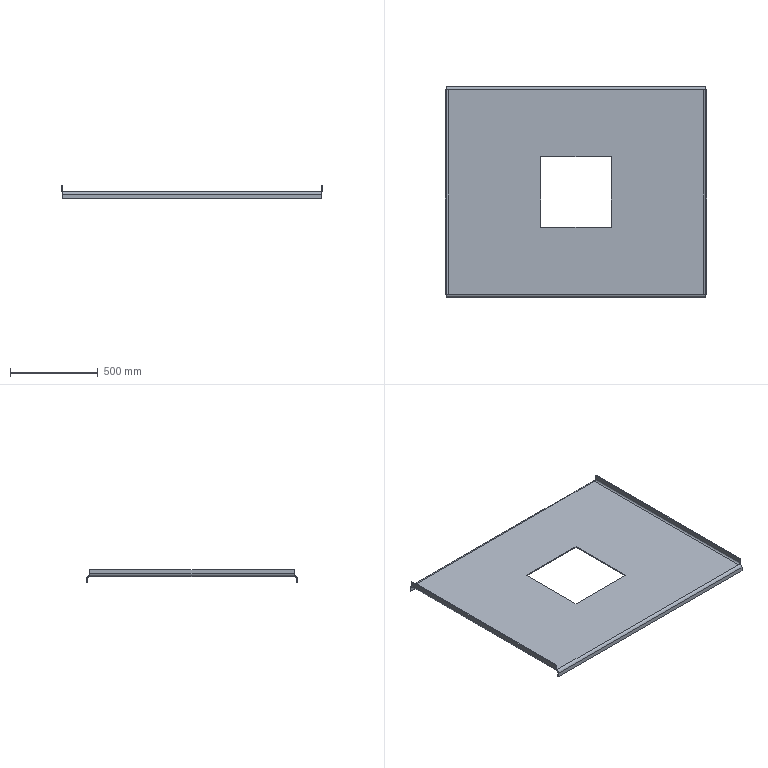Part | SolidWorks | features EdgeFlange 2, FlatPattern 1, ICE 1, SMBaseFlange 1, SheetMetal 1 | 1 solid | 46 faces | box 1492 x 1200 x 74 mm | volume 10683181 mm3 | plane 38 | cylinder 8 | commonest cylinder face diameters 20 x4 32 x4
STEP:
#1=CARTESIAN_POINT('',(740.,584.,-6.));
#2=VERTEX_POINT('',#1);
#3=CARTESIAN_POINT('',(740.,584.,-2.49));
#4=VERTEX_POINT('',#3);
#5=CARTESIAN_POINT('',(740.,584.,-6.));
#6=DIRECTION('',(0.,0.,1.));
#7=VECTOR('',#6,1000.);
#8=LINE('',#5,#7);
#9=EDGE_CURVE('',#2,#4,#8,.T.);
#10=ORIENTED_EDGE('',*,*,#9,.T.);
#11=CARTESIAN_POINT('',(730.,584.,-6.));
#12=VERTEX_POINT('',#11);
#13=CARTESIAN_POINT('',(730.,584.,10.));
#14=DIRECTION('',(0.,1.,0.));
#15=DIRECTION('',(0.,0.,1.));
#16=AXIS2_PLACEMENT_3D('',#13,#14,#15);
#17=CIRCLE('',#16,16.);
#18=EDGE_CURVE('',#4,#12,#17,.T.);
#19=ORIENTED_EDGE('',*,*,#18,.T.);
#20=CARTESIAN_POINT('',(740.,584.,-6.));
#21=DIRECTION('',(-1.,0.,0.));
#22=VECTOR('',#21,1000.);
#23=LINE('',#20,#22);
#24=EDGE_CURVE('',#2,#12,#23,.T.);
#25=ORIENTED_EDGE('',*,*,#24,.F.);
#26=EDGE_LOOP('',(#10,#19,#25));
#27=FACE_OUTER_BOUND('',#26,.T.);
#28=CARTESIAN_POINT('',(740.,584.,0.));
#29=DIRECTION('',(0.,-1.,0.));
#30=DIRECTION('',(1.,0.,0.));
#31=AXIS2_PLACEMENT_3D('',#28,#29,#30);
#32=PLANE('',#31);
#33=ADVANCED_FACE('',(#27),#32,.T.);
#34=CARTESIAN_POINT('',(730.,-584.,-6.));
#35=VERTEX_POINT('',#34);
#36=CARTESIAN_POINT('',(740.,-584.,-6.));
#37=VERTEX_POINT('',#36);
#38=CARTESIAN_POINT('',(-740.,-584.,-6.));
#39=DIRECTION('',(1.,0.,0.));
#40=VECTOR('',#39,1000.);
#41=LINE('',#38,#40);
#42=EDGE_CURVE('',#35,#37,#41,.T.);
#43=ORIENTED_EDGE('',*,*,#42,.F.);
#44=CARTESIAN_POINT('',(740.,-584.,-2.49));
#45=VERTEX_POINT('',#44);
#46=CARTESIAN_POINT('',(730.,-584.,10.));
#47=DIRECTION('',(0.,-1.,0.));
#48=DIRECTION('',(0.,0.,1.));
#49=AXIS2_PLACEMENT_3D('',#46,#47,#48);
#50=CIRCLE('',#49,16.);
#51=EDGE_CURVE('',#35,#45,#50,.T.);
#52=ORIENTED_EDGE('',*,*,#51,.T.);
#53=CARTESIAN_POINT('',(740.,-584.,-6.));
#54=DIRECTION('',(0.,0.,1.));
#55=VECTOR('',#54,1000.);
#56=LINE('',#53,#55);
#57=EDGE_CURVE('',#37,#45,#56,.T.);
#58=ORIENTED_EDGE('',*,*,#57,.F.);
#59=EDGE_LOOP('',(#43,#52,#58));
#60=FACE_OUTER_BOUND('',#59,.T.);
#61=CARTESIAN_POINT('',(730.,-584.,0.));
#62=DIRECTION('',(0.,1.,0.));
#63=DIRECTION('',(0.,0.,1.));
#64=AXIS2_PLACEMENT_3D('',#61,#62,#63);
#65=PLANE('',#64);
#66=ADVANCED_FACE('',(#60),#65,.T.);
#67=CARTESIAN_POINT('',(-740.,-584.,-6.));
#68=VERTEX_POINT('',#67);
#69=CARTESIAN_POINT('',(-740.,-584.,-2.49));
#70=VERTEX_POINT('',#69);
#71=CARTESIAN_POINT('',(-740.,-584.,-6.));
#72=DIRECTION('',(0.,0.,1.));
#73=VECTOR('',#72,1000.);
#74=LINE('',#71,#73);
#75=EDGE_CURVE('',#68,#70,#74,.T.);
#76=ORIENTED_EDGE('',*,*,#75,.T.);
#77=CARTESIAN_POINT('',(-730.,-584.,-6.));
#78=VERTEX_POINT('',#77);
#79=CARTESIAN_POINT('',(-730.,-584.,10.));
#80=DIRECTION('',(0.,-1.,0.));
#81=DIRECTION('',(0.,0.,-1.));
#82=AXIS2_PLACEMENT_3D('',#79,#80,#81);
#83=CIRCLE('',#82,16.);
#84=EDGE_CURVE('',#70,#78,#83,.T.);
#85=ORIENTED_EDGE('',*,*,#84,.T.);
#86=CARTESIAN_POINT('',(-740.,-584.,-6.));
#87=DIRECTION('',(1.,0.,0.));
#88=VECTOR('',#87,1000.);
#89=LINE('',#86,#88);
#90=EDGE_CURVE('',#68,#78,#89,.T.);
#91=ORIENTED_EDGE('',*,*,#90,.F.);
#92=EDGE_LOOP('',(#76,#85,#91));
#93=FACE_OUTER_BOUND('',#92,.T.);
#94=CARTESIAN_POINT('',(-740.,-584.,0.));
#95=DIRECTION('',(0.,1.,0.));
#96=DIRECTION('',(-1.,0.,0.));
#97=AXIS2_PLACEMENT_3D('',#94,#95,#96);
#98=PLANE('',#97);
#99=ADVANCED_FACE('',(#93),#98,.T.);
#100=CARTESIAN_POINT('',(-730.,584.,-6.));
#101=VERTEX_POINT('',#100);
#102=CARTESIAN_POINT('',(-740.,584.,-6.));
#103=VERTEX_POINT('',#102);
#104=CARTESIAN_POINT('',(740.,584.,-6.));
#105=DIRECTION('',(-1.,0.,0.));
#106=VECTOR('',#105,1000.);
#107=LINE('',#104,#106);
#108=EDGE_CURVE('',#101,#103,#107,.T.);
#109=ORIENTED_EDGE('',*,*,#108,.F.);
#110=CARTESIAN_POINT('',(-740.,584.,-2.49));
#111=VERTEX_POINT('',#110);
#112=CARTESIAN_POINT('',(-730.,584.,10.));
#113=DIRECTION('',(0.,1.,0.));
#114=DIRECTION('',(0.,0.,-1.));
#115=AXIS2_PLACEMENT_3D('',#112,#113,#114);
#116=CIRCLE('',#115,16.);
#117=EDGE_CURVE('',#101,#111,#116,.T.);
#118=ORIENTED_EDGE('',*,*,#117,.T.);
#119=CARTESIAN_POINT('',(-740.,584.,-6.));
#120=DIRECTION('',(0.,0.,1.));
#121=VECTOR('',#120,1000.);
#122=LINE('',#119,#121);
#123=EDGE_CURVE('',#103,#111,#122,.T.);
#124=ORIENTED_EDGE('',*,*,#123,.F.);
#125=EDGE_LOOP('',(#109,#118,#124));
#126=FACE_OUTER_BOUND('',#125,.T.);
#127=CARTESIAN_POINT('',(-730.,584.,0.));
#128=DIRECTION('',(0.,-1.,0.));
#129=DIRECTION('',(0.,0.,-1.));
#130=AXIS2_PLACEMENT_3D('',#127,#128,#129);
#131=PLANE('',#130);
#132=ADVANCED_FACE('',(#126),#131,.T.);
#133=CARTESIAN_POINT('',(-200.,200.,-6.));
#134=VERTEX_POINT('',#133);
#135=CARTESIAN_POINT('',(200.,200.,-6.));
#136=VERTEX_POINT('',#135);
#137=CARTESIAN_POINT('',(200.,200.,-6.));
#138=DIRECTION('',(1.,0.,0.));
#139=VECTOR('',#138,1000.);
#140=LINE('',#137,#139);
#141=EDGE_CURVE('',#134,#136,#140,.T.);
#142=ORIENTED_EDGE('',*,*,#141,.F.);
#143=CARTESIAN_POINT('',(-200.,-200.,-6.));
#144=VERTEX_POINT('',#143);
#145=CARTESIAN_POINT('',(-200.,-200.,-6.));
#146=DIRECTION('',(0.,1.,0.));
#147=VECTOR('',#146,1000.);
#148=LINE('',#145,#147);
#149=EDGE_CURVE('',#144,#134,#148,.T.);
#150=ORIENTED_EDGE('',*,*,#149,.F.);
#151=CARTESIAN_POINT('',(200.,-200.,-6.));
#152=VERTEX_POINT('',#151);
#153=CARTESIAN_POINT('',(200.,-200.,-6.));
#154=DIRECTION('',(-1.,0.,0.));
#155=VECTOR('',#154,1000.);
#156=LINE('',#153,#155);
#157=EDGE_CURVE('',#152,#144,#156,.T.);
#158=ORIENTED_EDGE('',*,*,#157,.F.);
#159=CARTESIAN_POINT('',(200.,-200.,-6.));
#160=DIRECTION('',(0.,-1.,0.));
#161=VECTOR('',#160,1000.);
#162=LINE('',#159,#161);
#163=EDGE_CURVE('',#136,#152,#162,.T.);
#164=ORIENTED_EDGE('',*,*,#163,.F.);
#165=EDGE_LOOP('',(#142,#150,#158,#164));
#166=FACE_BOUND('',#165,.T.);
#167=CARTESIAN_POINT('',(730.,584.,-6.));
#168=DIRECTION('',(0.,-1.,0.));
#169=VECTOR('',#168,1000.);
#170=LINE('',#167,#169);
#171=EDGE_CURVE('',#12,#35,#170,.T.);
#172=ORIENTED_EDGE('',*,*,#171,.T.);
#173=CARTESIAN_POINT('',(-740.,-584.,-6.));
#174=DIRECTION('',(1.,0.,0.));
#175=VECTOR('',#174,1000.);
#176=LINE('',#173,#175);
#177=EDGE_CURVE('',#78,#35,#176,.T.);
#178=ORIENTED_EDGE('',*,*,#177,.F.);
#179=CARTESIAN_POINT('',(-730.,-584.,-6.));
#180=DIRECTION('',(0.,1.,0.));
#181=VECTOR('',#180,1000.);
#182=LINE('',#179,#181);
#183=EDGE_CURVE('',#78,#101,#182,.T.);
#184=ORIENTED_EDGE('',*,*,#183,.T.);
#185=CARTESIAN_POINT('',(740.,584.,-6.));
#186=DIRECTION('',(-1.,0.,0.));
#187=VECTOR('',#186,1000.);
#188=LINE('',#185,#187);
#189=EDGE_CURVE('',#12,#101,#188,.T.);
#190=ORIENTED_EDGE('',*,*,#189,.F.);
#191=EDGE_LOOP('',(#172,#178,#184,#190));
#192=FACE_OUTER_BOUND('',#191,.T.);
#193=CARTESIAN_POINT('',(0.,0.,-6.));
#194=DIRECTION('',(0.,0.,1.));
#195=DIRECTION('',(1.,0.,0.));
#196=AXIS2_PLACEMENT_3D('',#193,#194,#195);
#197=PLANE('',#196);
#198=ADVANCED_FACE('',(#166,#192),#197,.F.);
#199=CARTESIAN_POINT('',(-200.,200.,0.));
#200=VERTEX_POINT('',#199);
#201=CARTESIAN_POINT('',(-200.,-200.,0.));
#202=VERTEX_POINT('',#201);
#203=CARTESIAN_POINT('',(-200.,0.,0.));
#204=DIRECTION('',(0.,-1.,0.));
#205=VECTOR('',#204,1000.);
#206=LINE('',#203,#205);
#207=EDGE_CURVE('',#200,#202,#206,.T.);
#208=ORIENTED_EDGE('',*,*,#207,.F.);
#209=CARTESIAN_POINT('',(200.,200.,0.));
#210=VERTEX_POINT('',#209);
#211=CARTESIAN_POINT('',(0.,200.,0.));
#212=DIRECTION('',(-1.,0.,0.));
#213=VECTOR('',#212,1000.);
#214=LINE('',#211,#213);
#215=EDGE_CURVE('',#210,#200,#214,.T.);
#216=ORIENTED_EDGE('',*,*,#215,.F.);
#217=CARTESIAN_POINT('',(200.,-200.,0.));
#218=VERTEX_POINT('',#217);
#219=CARTESIAN_POINT('',(200.,0.,0.));
#220=DIRECTION('',(0.,1.,0.));
#221=VECTOR('',#220,1000.);
#222=LINE('',#219,#221);
#223=EDGE_CURVE('',#218,#210,#222,.T.);
#224=ORIENTED_EDGE('',*,*,#223,.F.);
#225=CARTESIAN_POINT('',(0.,-200.,0.));
#226=DIRECTION('',(1.,0.,0.));
#227=VECTOR('',#226,1000.);
#228=LINE('',#225,#227);
#229=EDGE_CURVE('',#202,#218,#228,.T.);
#230=ORIENTED_EDGE('',*,*,#229,.F.);
#231=EDGE_LOOP('',(#208,#216,#224,#230));
#232=FACE_BOUND('',#231,.T.);
#233=CARTESIAN_POINT('',(-730.,-584.,0.));
#234=VERTEX_POINT('',#233);
#235=CARTESIAN_POINT('',(730.,-584.,0.));
#236=VERTEX_POINT('',#235);
#237=CARTESIAN_POINT('',(-740.,-584.,0.));
#238=DIRECTION('',(1.,0.,0.));
#239=VECTOR('',#238,1000.);
#240=LINE('',#237,#239);
#241=EDGE_CURVE('',#234,#236,#240,.T.);
#242=ORIENTED_EDGE('',*,*,#241,.T.);
#243=CARTESIAN_POINT('',(730.,584.,0.));
#244=VERTEX_POINT('',#243);
#245=CARTESIAN_POINT('',(730.,584.,0.));
#246=DIRECTION('',(0.,-1.,0.));
#247=VECTOR('',#246,1000.);
#248=LINE('',#245,#247);
#249=EDGE_CURVE('',#244,#236,#248,.T.);
#250=ORIENTED_EDGE('',*,*,#249,.F.);
#251=CARTESIAN_POINT('',(-730.,584.,0.));
#252=VERTEX_POINT('',#251);
#253=CARTESIAN_POINT('',(740.,584.,0.));
#254=DIRECTION('',(-1.,0.,0.));
#255=VECTOR('',#254,1000.);
#256=LINE('',#253,#255);
#257=EDGE_CURVE('',#244,#252,#256,.T.);
#258=ORIENTED_EDGE('',*,*,#257,.T.);
#259=CARTESIAN_POINT('',(-730.,-584.,0.));
#260=DIRECTION('',(0.,1.,0.));
#261=VECTOR('',#260,1000.);
#262=LINE('',#259,#261);
#263=EDGE_CURVE('',#234,#252,#262,.T.);
#264=ORIENTED_EDGE('',*,*,#263,.F.);
#265=EDGE_LOOP('',(#242,#250,#258,#264));
#266=FACE_OUTER_BOUND('',#265,.T.);
#267=CARTESIAN_POINT('',(0.,0.,0.));
#268=DIRECTION('',(0.,0.,1.));
#269=DIRECTION('',(1.,0.,0.));
#270=AXIS2_PLACEMENT_3D('',#267,#268,#269);
#271=PLANE('',#270);
#272=ADVANCED_FACE('',(#232,#266),#271,.T.);
#273=CARTESIAN_POINT('',(740.,-594.,-16.));
#274=VERTEX_POINT('',#273);
#275=CARTESIAN_POINT('',(740.,-600.,-16.));
#276=VERTEX_POINT('',#275);
#277=CARTESIAN_POINT('',(740.,-600.,-16.));
#278=DIRECTION('',(0.,-1.,0.));
#279=VECTOR('',#278,1000.);
#280=LINE('',#277,#279);
#281=EDGE_CURVE('',#274,#276,#280,.T.);
#282=ORIENTED_EDGE('',*,*,#281,.F.);
#283=CARTESIAN_POINT('',(740.,-584.,-16.));
#284=DIRECTION('',(1.,0.,0.));
#285=DIRECTION('',(0.,0.,1.));
#286=AXIS2_PLACEMENT_3D('',#283,#284,#285);
#287=CIRCLE('',#286,10.);
#288=EDGE_CURVE('',#37,#274,#287,.T.);
#289=ORIENTED_EDGE('',*,*,#288,.F.);
#290=ORIENTED_EDGE('',*,*,#57,.T.);
#291=CARTESIAN_POINT('',(740.,-584.,0.));
#292=VERTEX_POINT('',#291);
#293=CARTESIAN_POINT('',(740.,-584.,-6.));
#294=DIRECTION('',(0.,0.,1.));
#295=VECTOR('',#294,1000.);
#296=LINE('',#293,#295);
#297=EDGE_CURVE('',#45,#292,#296,.T.);
#298=ORIENTED_EDGE('',*,*,#297,.T.);
#299=CARTESIAN_POINT('',(740.,-584.,-16.));
#300=DIRECTION('',(1.,0.,0.));
#301=DIRECTION('',(0.,0.,1.));
#302=AXIS2_PLACEMENT_3D('',#299,#300,#301);
#303=CIRCLE('',#302,16.);
#304=EDGE_CURVE('',#292,#276,#303,.T.);
#305=ORIENTED_EDGE('',*,*,#304,.T.);
#306=EDGE_LOOP('',(#282,#289,#290,#298,#305));
#307=FACE_OUTER_BOUND('',#306,.T.);
#308=CARTESIAN_POINT('',(740.,-584.,-16.));
#309=DIRECTION('',(1.,0.,0.));
#310=DIRECTION('',(0.,0.,-1.));
#311=AXIS2_PLACEMENT_3D('',#308,#309,#310);
#312=PLANE('',#311);
#313=ADVANCED_FACE('',(#307),#312,.T.);
#314=CARTESIAN_POINT('',(-740.,-594.,-16.));
#315=VERTEX_POINT('',#314);
#316=CARTESIAN_POINT('',(-740.,-584.,-16.));
#317=DIRECTION('',(-1.,0.,0.));
#318=DIRECTION('',(0.,0.,1.));
#319=AXIS2_PLACEMENT_3D('',#316,#317,#318);
#320=CIRCLE('',#319,10.);
#321=EDGE_CURVE('',#315,#68,#320,.T.);
#322=ORIENTED_EDGE('',*,*,#321,.F.);
#323=CARTESIAN_POINT('',(-740.,-600.,-16.));
#324=VERTEX_POINT('',#323);
#325=CARTESIAN_POINT('',(-740.,-594.,-16.));
#326=DIRECTION('',(0.,-1.,0.));
#327=VECTOR('',#326,1000.);
#328=LINE('',#325,#327);
#329=EDGE_CURVE('',#315,#324,#328,.T.);
#330=ORIENTED_EDGE('',*,*,#329,.T.);
#331=CARTESIAN_POINT('',(-740.,-584.,0.));
#332=VERTEX_POINT('',#331);
#333=CARTESIAN_POINT('',(-740.,-584.,-16.));
#334=DIRECTION('',(-1.,0.,0.));
#335=DIRECTION('',(0.,0.,1.));
#336=AXIS2_PLACEMENT_3D('',#333,#334,#335);
#337=CIRCLE('',#336,16.);
#338=EDGE_CURVE('',#324,#332,#337,.T.);
#339=ORIENTED_EDGE('',*,*,#338,.T.);
#340=CARTESIAN_POINT('',(-740.,-584.,-6.));
#341=DIRECTION('',(0.,0.,1.));
#342=VECTOR('',#341,1000.);
#343=LINE('',#340,#342);
#344=EDGE_CURVE('',#70,#332,#343,.T.);
#345=ORIENTED_EDGE('',*,*,#344,.F.);
#346=ORIENTED_EDGE('',*,*,#75,.F.);
#347=EDGE_LOOP('',(#322,#330,#339,#345,#346));
#348=FACE_OUTER_BOUND('',#347,.T.);
#349=CARTESIAN_POINT('',(-740.,-584.,-16.));
#350=DIRECTION('',(1.,0.,0.));
#351=DIRECTION('',(0.,0.,-1.));
#352=AXIS2_PLACEMENT_3D('',#349,#350,#351);
#353=PLANE('',#352);
#354=ADVANCED_FACE('',(#348),#353,.F.);
#355=CARTESIAN_POINT('',(-740.,-584.,0.));
#356=DIRECTION('',(1.,0.,0.));
#357=VECTOR('',#356,1000.);
#358=LINE('',#355,#357);
#359=EDGE_CURVE('',#332,#234,#358,.T.);
#360=ORIENTED_EDGE('',*,*,#359,.F.);
#361=ORIENTED_EDGE('',*,*,#338,.F.);
#362=CARTESIAN_POINT('',(740.,-600.,-16.));
#363=DIRECTION('',(1.,0.,0.));
#364=VECTOR('',#363,1000.);
#365=LINE('',#362,#364);
#366=EDGE_CURVE('',#324,#276,#365,.T.);
#367=ORIENTED_EDGE('',*,*,#366,.T.);
#368=ORIENTED_EDGE('',*,*,#304,.F.);
#369=CARTESIAN_POINT('',(730.,-584.,0.));
#370=DIRECTION('',(1.,0.,0.));
#371=VECTOR('',#370,1000.);
#372=LINE('',#369,#371);
#373=EDGE_CURVE('',#236,#292,#372,.T.);
#374=ORIENTED_EDGE('',*,*,#373,.F.);
#375=ORIENTED_EDGE('',*,*,#241,.F.);
#376=EDGE_LOOP('',(#360,#361,#367,#368,#374,#375));
#377=FACE_OUTER_BOUND('',#376,.T.);
#378=CARTESIAN_POINT('',(-740.,-584.,-16.));
#379=DIRECTION('',(-1.,0.,0.));
#380=DIRECTION('',(0.,-1.,0.));
#381=AXIS2_PLACEMENT_3D('',#378,#379,#380);
#382=CYLINDRICAL_SURFACE('',#381,16.);
#383=ADVANCED_FACE('',(#377),#382,.T.);
#384=ORIENTED_EDGE('',*,*,#90,.T.);
#385=ORIENTED_EDGE('',*,*,#177,.T.);
#386=ORIENTED_EDGE('',*,*,#42,.T.);
#387=ORIENTED_EDGE('',*,*,#288,.T.);
#388=CARTESIAN_POINT('',(740.,-594.,-16.));
#389=DIRECTION('',(-1.,0.,0.));
#390=VECTOR('',#389,1000.);
#391=LINE('',#388,#390);
#392=EDGE_CURVE('',#274,#315,#391,.T.);
#393=ORIENTED_EDGE('',*,*,#392,.T.);
#394=ORIENTED_EDGE('',*,*,#321,.T.);
#395=EDGE_LOOP('',(#384,#385,#386,#387,#393,#394));
#396=FACE_OUTER_BOUND('',#395,.T.);
#397=CARTESIAN_POINT('',(-740.,-584.,-16.));
#398=DIRECTION('',(-1.,0.,0.));
#399=DIRECTION('',(0.,-1.,0.));
#400=AXIS2_PLACEMENT_3D('',#397,#398,#399);
#401=CYLINDRICAL_SURFACE('',#400,10.);
#402=ADVANCED_FACE('',(#396),#401,.F.);
#403=ORIENTED_EDGE('',*,*,#329,.F.);
#404=CARTESIAN_POINT('',(-740.,-594.,-40.));
#405=VERTEX_POINT('',#404);
#406=CARTESIAN_POINT('',(-740.,-594.,-40.));
#407=DIRECTION('',(0.,0.,-1.));
#408=VECTOR('',#407,1000.);
#409=LINE('',#406,#408);
#410=EDGE_CURVE('',#315,#405,#409,.T.);
#411=ORIENTED_EDGE('',*,*,#410,.T.);
#412=CARTESIAN_POINT('',(-740.,-600.,-40.));
#413=VERTEX_POINT('',#412);
#414=CARTESIAN_POINT('',(-740.,-600.,-40.));
#415=DIRECTION('',(0.,1.,0.));
#416=VECTOR('',#415,1000.);
#417=LINE('',#414,#416);
#418=EDGE_CURVE('',#413,#405,#417,.T.);
#419=ORIENTED_EDGE('',*,*,#418,.F.);
#420=CARTESIAN_POINT('',(-740.,-600.,0.));
#421=DIRECTION('',(0.,0.,-1.));
#422=VECTOR('',#421,1000.);
#423=LINE('',#420,#422);
#424=EDGE_CURVE('',#324,#413,#423,.T.);
#425=ORIENTED_EDGE('',*,*,#424,.F.);
#426=EDGE_LOOP('',(#403,#411,#419,#425));
#427=FACE_OUTER_BOUND('',#426,.T.);
#428=CARTESIAN_POINT('',(-740.,-600.,-40.));
#429=DIRECTION('',(1.,0.,0.));
#430=DIRECTION('',(0.,0.,-1.));
#431=AXIS2_PLACEMENT_3D('',#428,#429,#430);
#432=PLANE('',#431);
#433=ADVANCED_FACE('',(#427),#432,.F.);
#434=ORIENTED_EDGE('',*,*,#281,.T.);
#435=CARTESIAN_POINT('',(740.,-600.,-40.));
#436=VERTEX_POINT('',#435);
#437=CARTESIAN_POINT('',(740.,-600.,0.));
#438=DIRECTION('',(0.,0.,1.));
#439=VECTOR('',#438,1000.);
#440=LINE('',#437,#439);
#441=EDGE_CURVE('',#436,#276,#440,.T.);
#442=ORIENTED_EDGE('',*,*,#441,.F.);
#443=CARTESIAN_POINT('',(740.,-594.,-40.));
#444=VERTEX_POINT('',#443);
#445=CARTESIAN_POINT('',(740.,-600.,-40.));
#446=DIRECTION('',(0.,1.,0.));
#447=VECTOR('',#446,1000.);
#448=LINE('',#445,#447);
#449=EDGE_CURVE('',#436,#444,#448,.T.);
#450=ORIENTED_EDGE('',*,*,#449,.T.);
#451=CARTESIAN_POINT('',(740.,-594.,-6.));
#452=DIRECTION('',(0.,0.,1.));
#453=VECTOR('',#452,1000.);
#454=LINE('',#451,#453);
#455=EDGE_CURVE('',#444,#274,#454,.T.);
#456=ORIENTED_EDGE('',*,*,#455,.T.);
#457=EDGE_LOOP('',(#434,#442,#450,#456));
#458=FACE_OUTER_BOUND('',#457,.T.);
#459=CARTESIAN_POINT('',(740.,-600.,-6.));
#460=DIRECTION('',(-1.,0.,0.));
#461=DIRECTION('',(0.,0.,1.));
#462=AXIS2_PLACEMENT_3D('',#459,#460,#461);
#463=PLANE('',#462);
#464=ADVANCED_FACE('',(#458),#463,.F.);
#465=ORIENTED_EDGE('',*,*,#366,.F.);
#466=ORIENTED_EDGE('',*,*,#424,.T.);
#467=CARTESIAN_POINT('',(0.,-600.,-40.));
#468=DIRECTION('',(1.,0.,0.));
#469=VECTOR('',#468,1000.);
#470=LINE('',#467,#469);
#471=EDGE_CURVE('',#413,#436,#470,.T.);
#472=ORIENTED_EDGE('',*,*,#471,.T.);
#473=ORIENTED_EDGE('',*,*,#441,.T.);
#474=EDGE_LOOP('',(#465,#466,#472,#473));
#475=FACE_OUTER_BOUND('',#474,.T.);
#476=CARTESIAN_POINT('',(0.,-600.,0.));
#477=DIRECTION('',(0.,1.,0.));
#478=DIRECTION('',(0.,0.,1.));
#479=AXIS2_PLACEMENT_3D('',#476,#477,#478);
#480=PLANE('',#479);
#481=ADVANCED_FACE('',(#475),#480,.F.);
#482=ORIENTED_EDGE('',*,*,#410,.F.);
#483=ORIENTED_EDGE('',*,*,#392,.F.);
#484=ORIENTED_EDGE('',*,*,#455,.F.);
#485=CARTESIAN_POINT('',(740.,-594.,-40.));
#486=DIRECTION('',(1.,0.,0.));
#487=VECTOR('',#486,1000.);
#488=LINE('',#485,#487);
#489=EDGE_CURVE('',#405,#444,#488,.T.);
#490=ORIENTED_EDGE('',*,*,#489,.F.);
#491=EDGE_LOOP('',(#482,#483,#484,#490));
#492=FACE_OUTER_BOUND('',#491,.T.);
#493=CARTESIAN_POINT('',(0.,-594.,0.));
#494=DIRECTION('',(0.,1.,0.));
#495=DIRECTION('',(0.,0.,1.));
#496=AXIS2_PLACEMENT_3D('',#493,#494,#495);
#497=PLANE('',#496);
#498=ADVANCED_FACE('',(#492),#497,.T.);
#499=ORIENTED_EDGE('',*,*,#489,.T.);
#500=ORIENTED_EDGE('',*,*,#449,.F.);
#501=ORIENTED_EDGE('',*,*,#471,.F.);
#502=ORIENTED_EDGE('',*,*,#418,.T.);
#503=EDGE_LOOP('',(#499,#500,#501,#502));
#504=FACE_OUTER_BOUND('',#503,.T.);
#505=CARTESIAN_POINT('',(740.,-600.,-40.));
#506=DIRECTION('',(0.,0.,1.));
#507=DIRECTION('',(0.,-1.,0.));
#508=AXIS2_PLACEMENT_3D('',#505,#506,#507);
#509=PLANE('',#508);
#510=ADVANCED_FACE('',(#504),#509,.F.);
#511=CARTESIAN_POINT('',(-740.,594.,-16.));
#512=VERTEX_POINT('',#511);
#513=CARTESIAN_POINT('',(-740.,600.,-16.));
#514=VERTEX_POINT('',#513);
#515=CARTESIAN_POINT('',(-740.,600.,-16.));
#516=DIRECTION('',(0.,1.,0.));
#517=VECTOR('',#516,1000.);
#518=LINE('',#515,#517);
#519=EDGE_CURVE('',#512,#514,#518,.T.);
#520=ORIENTED_EDGE('',*,*,#519,.F.);
#521=CARTESIAN_POINT('',(-740.,584.,-16.));
#522=DIRECTION('',(-1.,0.,0.));
#523=DIRECTION('',(0.,0.,-1.));
#524=AXIS2_PLACEMENT_3D('',#521,#522,#523);
#525=CIRCLE('',#524,10.);
#526=EDGE_CURVE('',#103,#512,#525,.T.);
#527=ORIENTED_EDGE('',*,*,#526,.F.);
#528=ORIENTED_EDGE('',*,*,#123,.T.);
#529=CARTESIAN_POINT('',(-740.,584.,0.));
#530=VERTEX_POINT('',#529);
#531=CARTESIAN_POINT('',(-740.,584.,-6.));
#532=DIRECTION('',(0.,0.,1.));
#533=VECTOR('',#532,1000.);
#534=LINE('',#531,#533);
#535=EDGE_CURVE('',#111,#530,#534,.T.);
#536=ORIENTED_EDGE('',*,*,#535,.T.);
#537=CARTESIAN_POINT('',(-740.,584.,-16.));
#538=DIRECTION('',(-1.,0.,0.));
#539=DIRECTION('',(0.,0.,-1.));
#540=AXIS2_PLACEMENT_3D('',#537,#538,#539);
#541=CIRCLE('',#540,16.);
#542=EDGE_CURVE('',#530,#514,#541,.T.);
#543=ORIENTED_EDGE('',*,*,#542,.T.);
#544=EDGE_LOOP('',(#520,#527,#528,#536,#543));
#545=FACE_OUTER_BOUND('',#544,.T.);
#546=CARTESIAN_POINT('',(-740.,584.,-16.));
#547=DIRECTION('',(-1.,0.,0.));
#548=DIRECTION('',(0.,0.,1.));
#549=AXIS2_PLACEMENT_3D('',#546,#547,#548);
#550=PLANE('',#549);
#551=ADVANCED_FACE('',(#545),#550,.T.);
#552=CARTESIAN_POINT('',(740.,594.,-16.));
#553=VERTEX_POINT('',#552);
#554=CARTESIAN_POINT('',(740.,584.,-16.));
#555=DIRECTION('',(1.,0.,0.));
#556=DIRECTION('',(0.,0.,-1.));
#557=AXIS2_PLACEMENT_3D('',#554,#555,#556);
#558=CIRCLE('',#557,10.);
#559=EDGE_CURVE('',#553,#2,#558,.T.);
#560=ORIENTED_EDGE('',*,*,#559,.F.);
#561=CARTESIAN_POINT('',(740.,600.,-16.));
#562=VERTEX_POINT('',#561);
#563=CARTESIAN_POINT('',(740.,594.,-16.));
#564=DIRECTION('',(0.,1.,0.));
#565=VECTOR('',#564,1000.);
#566=LINE('',#563,#565);
#567=EDGE_CURVE('',#553,#562,#566,.T.);
#568=ORIENTED_EDGE('',*,*,#567,.T.);
#569=CARTESIAN_POINT('',(740.,584.,0.));
#570=VERTEX_POINT('',#569);
#571=CARTESIAN_POINT('',(740.,584.,-16.));
#572=DIRECTION('',(1.,0.,0.));
#573=DIRECTION('',(0.,0.,-1.));
#574=AXIS2_PLACEMENT_3D('',#571,#572,#573);
#575=CIRCLE('',#574,16.);
#576=EDGE_CURVE('',#562,#570,#575,.T.);
#577=ORIENTED_EDGE('',*,*,#576,.T.);
#578=CARTESIAN_POINT('',(740.,584.,-6.));
#579=DIRECTION('',(0.,0.,1.));
#580=VECTOR('',#579,1000.);
#581=LINE('',#578,#580);
#582=EDGE_CURVE('',#4,#570,#581,.T.);
#583=ORIENTED_EDGE('',*,*,#582,.F.);
#584=ORIENTED_EDGE('',*,*,#9,.F.);
#585=EDGE_LOOP('',(#560,#568,#577,#583,#584));
#586=FACE_OUTER_BOUND('',#585,.T.);
#587=CARTESIAN_POINT('',(740.,584.,-16.));
#588=DIRECTION('',(-1.,0.,0.));
#589=DIRECTION('',(0.,0.,1.));
#590=AXIS2_PLACEMENT_3D('',#587,#588,#589);
#591=PLANE('',#590);
#592=ADVANCED_FACE('',(#586),#591,.F.);
#593=CARTESIAN_POINT('',(740.,584.,0.));
#594=DIRECTION('',(-1.,0.,0.));
#595=VECTOR('',#594,1000.);
#596=LINE('',#593,#595);
#597=EDGE_CURVE('',#570,#244,#596,.T.);
#598=ORIENTED_EDGE('',*,*,#597,.F.);
#599=ORIENTED_EDGE('',*,*,#576,.F.);
#600=CARTESIAN_POINT('',(0.,600.,-16.));
#601=DIRECTION('',(1.,0.,0.));
#602=VECTOR('',#601,1000.);
#603=LINE('',#600,#602);
#604=EDGE_CURVE('',#514,#562,#603,.T.);
#605=ORIENTED_EDGE('',*,*,#604,.F.);
#606=ORIENTED_EDGE('',*,*,#542,.F.);
#607=CARTESIAN_POINT('',(-730.,584.,0.));
#608=DIRECTION('',(-1.,0.,0.));
#609=VECTOR('',#608,1000.);
#610=LINE('',#607,#609);
#611=EDGE_CURVE('',#252,#530,#610,.T.);
#612=ORIENTED_EDGE('',*,*,#611,.F.);
#613=ORIENTED_EDGE('',*,*,#257,.F.);
#614=EDGE_LOOP('',(#598,#599,#605,#606,#612,#613));
#615=FACE_OUTER_BOUND('',#614,.T.);
#616=CARTESIAN_POINT('',(740.,584.,-16.));
#617=DIRECTION('',(1.,0.,0.));
#618=DIRECTION('',(0.,1.,0.));
#619=AXIS2_PLACEMENT_3D('',#616,#617,#618);
#620=CYLINDRICAL_SURFACE('',#619,16.);
#621=ADVANCED_FACE('',(#615),#620,.T.);
#622=ORIENTED_EDGE('',*,*,#24,.T.);
#623=ORIENTED_EDGE('',*,*,#189,.T.);
#624=ORIENTED_EDGE('',*,*,#108,.T.);
#625=ORIENTED_EDGE('',*,*,#526,.T.);
#626=CARTESIAN_POINT('',(-740.,594.,-16.));
#627=DIRECTION('',(1.,0.,0.));
#628=VECTOR('',#627,1000.);
#629=LINE('',#626,#628);
#630=EDGE_CURVE('',#512,#553,#629,.T.);
#631=ORIENTED_EDGE('',*,*,#630,.T.);
#632=ORIENTED_EDGE('',*,*,#559,.T.);
#633=EDGE_LOOP('',(#622,#623,#624,#625,#631,#632));
#634=FACE_OUTER_BOUND('',#633,.T.);
#635=CARTESIAN_POINT('',(740.,584.,-16.));
#636=DIRECTION('',(1.,0.,0.));
#637=DIRECTION('',(0.,1.,0.));
#638=AXIS2_PLACEMENT_3D('',#635,#636,#637);
#639=CYLINDRICAL_SURFACE('',#638,10.);
#640=ADVANCED_FACE('',(#634),#639,.F.);
#641=ORIENTED_EDGE('',*,*,#567,.F.);
#642=CARTESIAN_POINT('',(740.,594.,-40.));
#643=VERTEX_POINT('',#642);
#644=CARTESIAN_POINT('',(740.,594.,-6.));
#645=DIRECTION('',(0.,0.,-1.));
#646=VECTOR('',#645,1000.);
#647=LINE('',#644,#646);
#648=EDGE_CURVE('',#553,#643,#647,.T.);
#649=ORIENTED_EDGE('',*,*,#648,.T.);
#650=CARTESIAN_POINT('',(740.,600.,-40.));
#651=VERTEX_POINT('',#650);
#652=CARTESIAN_POINT('',(740.,600.,-40.));
#653=DIRECTION('',(0.,-1.,0.));
#654=VECTOR('',#653,1000.);
#655=LINE('',#652,#654);
#656=EDGE_CURVE('',#651,#643,#655,.T.);
#657=ORIENTED_EDGE('',*,*,#656,.F.);
#658=CARTESIAN_POINT('',(740.,600.,0.));
#659=DIRECTION('',(0.,0.,-1.));
#660=VECTOR('',#659,1000.);
#661=LINE('',#658,#660);
#662=EDGE_CURVE('',#562,#651,#661,.T.);
#663=ORIENTED_EDGE('',*,*,#662,.F.);
#664=EDGE_LOOP('',(#641,#649,#657,#663));
#665=FACE_OUTER_BOUND('',#664,.T.);
#666=CARTESIAN_POINT('',(740.,600.,-6.));
#667=DIRECTION('',(-1.,0.,0.));
#668=DIRECTION('',(0.,0.,1.));
#669=AXIS2_PLACEMENT_3D('',#666,#667,#668);
#670=PLANE('',#669);
#671=ADVANCED_FACE('',(#665),#670,.F.);
#672=ORIENTED_EDGE('',*,*,#519,.T.);
#673=CARTESIAN_POINT('',(-740.,600.,-40.));
#674=VERTEX_POINT('',#673);
#675=CARTESIAN_POINT('',(-740.,600.,0.));
#676=DIRECTION('',(0.,0.,1.));
#677=VECTOR('',#676,1000.);
#678=LINE('',#675,#677);
#679=EDGE_CURVE('',#674,#514,#678,.T.);
#680=ORIENTED_EDGE('',*,*,#679,.F.);
#681=CARTESIAN_POINT('',(-740.,594.,-40.));
#682=VERTEX_POINT('',#681);
#683=CARTESIAN_POINT('',(-740.,600.,-40.));
#684=DIRECTION('',(0.,-1.,0.));
#685=VECTOR('',#684,1000.);
#686=LINE('',#683,#685);
#687=EDGE_CURVE('',#674,#682,#686,.T.);
#688=ORIENTED_EDGE('',*,*,#687,.T.);
#689=CARTESIAN_POINT('',(-740.,594.,-40.));
#690=DIRECTION('',(0.,0.,1.));
#691=VECTOR('',#690,1000.);
#692=LINE('',#689,#691);
#693=EDGE_CURVE('',#682,#512,#692,.T.);
#694=ORIENTED_EDGE('',*,*,#693,.T.);
#695=EDGE_LOOP('',(#672,#680,#688,#694));
#696=FACE_OUTER_BOUND('',#695,.T.);
#697=CARTESIAN_POINT('',(-740.,600.,-40.));
#698=DIRECTION('',(1.,0.,0.));
#699=DIRECTION('',(0.,0.,-1.));
#700=AXIS2_PLACEMENT_3D('',#697,#698,#699);
#701=PLANE('',#700);
#702=ADVANCED_FACE('',(#696),#701,.F.);
#703=ORIENTED_EDGE('',*,*,#679,.T.);
#704=ORIENTED_EDGE('',*,*,#604,.T.);
#705=ORIENTED_EDGE('',*,*,#662,.T.);
#706=CARTESIAN_POINT('',(0.,600.,-40.));
#707=DIRECTION('',(-1.,0.,0.));
#708=VECTOR('',#707,1000.);
#709=LINE('',#706,#708);
#710=EDGE_CURVE('',#651,#674,#709,.T.);
#711=ORIENTED_EDGE('',*,*,#710,.T.);
#712=EDGE_LOOP('',(#703,#704,#705,#711));
#713=FACE_OUTER_BOUND('',#712,.T.);
#714=CARTESIAN_POINT('',(0.,600.,0.));
#715=DIRECTION('',(0.,1.,0.));
#716=DIRECTION('',(0.,0.,1.));
#717=AXIS2_PLACEMENT_3D('',#714,#715,#716);
#718=PLANE('',#717);
#719=ADVANCED_FACE('',(#713),#718,.T.);
#720=ORIENTED_EDGE('',*,*,#630,.F.);
#721=ORIENTED_EDGE('',*,*,#693,.F.);
#722=CARTESIAN_POINT('',(740.,594.,-40.));
#723=DIRECTION('',(-1.,0.,0.));
#724=VECTOR('',#723,1000.);
#725=LINE('',#722,#724);
#726=EDGE_CURVE('',#643,#682,#725,.T.);
#727=ORIENTED_EDGE('',*,*,#726,.F.);
#728=ORIENTED_EDGE('',*,*,#648,.F.);
#729=EDGE_LOOP('',(#720,#721,#727,#728));
#730=FACE_OUTER_BOUND('',#729,.T.);
#731=CARTESIAN_POINT('',(0.,594.,0.));
#732=DIRECTION('',(0.,1.,0.));
#733=DIRECTION('',(0.,0.,1.));
#734=AXIS2_PLACEMENT_3D('',#731,#732,#733);
#735=PLANE('',#734);
#736=ADVANCED_FACE('',(#730),#735,.F.);
#737=ORIENTED_EDGE('',*,*,#726,.T.);
#738=ORIENTED_EDGE('',*,*,#687,.F.);
#739=ORIENTED_EDGE('',*,*,#710,.F.);
#740=ORIENTED_EDGE('',*,*,#656,.T.);
#741=EDGE_LOOP('',(#737,#738,#739,#740));
#742=FACE_OUTER_BOUND('',#741,.T.);
#743=CARTESIAN_POINT('',(740.,600.,-40.));
#744=DIRECTION('',(0.,0.,1.));
#745=DIRECTION('',(0.,-1.,0.));
#746=AXIS2_PLACEMENT_3D('',#743,#744,#745);
#747=PLANE('',#746);
#748=ADVANCED_FACE('',(#742),#747,.F.);
#749=ORIENTED_EDGE('',*,*,#535,.F.);
#750=CARTESIAN_POINT('',(-746.,584.,10.));
#751=VERTEX_POINT('',#750);
#752=CARTESIAN_POINT('',(-730.,584.,10.));
#753=DIRECTION('',(0.,1.,0.));
#754=DIRECTION('',(0.,0.,-1.));
#755=AXIS2_PLACEMENT_3D('',#752,#753,#754);
#756=CIRCLE('',#755,16.);
#757=EDGE_CURVE('',#111,#751,#756,.T.);
#758=ORIENTED_EDGE('',*,*,#757,.T.);
#759=CARTESIAN_POINT('',(-740.,584.,10.));
#760=VERTEX_POINT('',#759);
#761=CARTESIAN_POINT('',(-740.,584.,10.));
#762=DIRECTION('',(-1.,0.,0.));
#763=VECTOR('',#762,1000.);
#764=LINE('',#761,#763);
#765=EDGE_CURVE('',#760,#751,#764,.T.);
#766=ORIENTED_EDGE('',*,*,#765,.F.);
#767=CARTESIAN_POINT('',(-730.,584.,10.));
#768=DIRECTION('',(0.,1.,0.));
#769=DIRECTION('',(0.,0.,-1.));
#770=AXIS2_PLACEMENT_3D('',#767,#768,#769);
#771=CIRCLE('',#770,10.);
#772=EDGE_CURVE('',#252,#760,#771,.T.);
#773=ORIENTED_EDGE('',*,*,#772,.F.);
#774=ORIENTED_EDGE('',*,*,#611,.T.);
#775=EDGE_LOOP('',(#749,#758,#766,#773,#774));
#776=FACE_OUTER_BOUND('',#775,.T.);
#777=CARTESIAN_POINT('',(-730.,584.,10.));
#778=DIRECTION('',(0.,1.,0.));
#779=DIRECTION('',(0.,0.,1.));
#780=AXIS2_PLACEMENT_3D('',#777,#778,#779);
#781=PLANE('',#780);
#782=ADVANCED_FACE('',(#776),#781,.T.);
#783=CARTESIAN_POINT('',(-746.,-584.,10.));
#784=VERTEX_POINT('',#783);
#785=CARTESIAN_POINT('',(-730.,-584.,10.));
#786=DIRECTION('',(0.,-1.,0.));
#787=DIRECTION('',(0.,0.,-1.));
#788=AXIS2_PLACEMENT_3D('',#785,#786,#787);
#789=CIRCLE('',#788,16.);
#790=EDGE_CURVE('',#784,#70,#789,.T.);
#791=ORIENTED_EDGE('',*,*,#790,.T.);
#792=ORIENTED_EDGE('',*,*,#344,.T.);
#793=ORIENTED_EDGE('',*,*,#359,.T.);
#794=CARTESIAN_POINT('',(-740.,-584.,10.));
#795=VERTEX_POINT('',#794);
#796=CARTESIAN_POINT('',(-730.,-584.,10.));
#797=DIRECTION('',(0.,-1.,0.));
#798=DIRECTION('',(0.,0.,-1.));
#799=AXIS2_PLACEMENT_3D('',#796,#797,#798);
#800=CIRCLE('',#799,10.);
#801=EDGE_CURVE('',#795,#234,#800,.T.);
#802=ORIENTED_EDGE('',*,*,#801,.F.);
#803=CARTESIAN_POINT('',(-740.,-584.,10.));
#804=DIRECTION('',(-1.,0.,0.));
#805=VECTOR('',#804,1000.);
#806=LINE('',#803,#805);
#807=EDGE_CURVE('',#795,#784,#806,.T.);
#808=ORIENTED_EDGE('',*,*,#807,.T.);
#809=EDGE_LOOP('',(#791,#792,#793,#802,#808));
#810=FACE_OUTER_BOUND('',#809,.T.);
#811=CARTESIAN_POINT('',(-730.,-584.,10.));
#812=DIRECTION('',(0.,1.,0.));
#813=DIRECTION('',(0.,0.,1.));
#814=AXIS2_PLACEMENT_3D('',#811,#812,#813);
#815=PLANE('',#814);
#816=ADVANCED_FACE('',(#810),#815,.F.);
#817=ORIENTED_EDGE('',*,*,#183,.F.);
#818=ORIENTED_EDGE('',*,*,#84,.F.);
#819=ORIENTED_EDGE('',*,*,#790,.F.);
#820=CARTESIAN_POINT('',(-746.,0.,10.));
#821=DIRECTION('',(0.,-1.,0.));
#822=VECTOR('',#821,1000.);
#823=LINE('',#820,#822);
#824=EDGE_CURVE('',#751,#784,#823,.T.);
#825=ORIENTED_EDGE('',*,*,#824,.F.);
#826=ORIENTED_EDGE('',*,*,#757,.F.);
#827=ORIENTED_EDGE('',*,*,#117,.F.);
#828=EDGE_LOOP('',(#817,#818,#819,#825,#826,#827));
#829=FACE_OUTER_BOUND('',#828,.T.);
#830=CARTESIAN_POINT('',(-730.,-584.,10.));
#831=DIRECTION('',(0.,-1.,0.));
#832=DIRECTION('',(-1.,0.,0.));
#833=AXIS2_PLACEMENT_3D('',#830,#831,#832);
#834=CYLINDRICAL_SURFACE('',#833,16.);
#835=ADVANCED_FACE('',(#829),#834,.T.);
#836=ORIENTED_EDGE('',*,*,#263,.T.);
#837=ORIENTED_EDGE('',*,*,#772,.T.);
#838=CARTESIAN_POINT('',(-740.,584.,10.));
#839=DIRECTION('',(0.,-1.,0.));
#840=VECTOR('',#839,1000.);
#841=LINE('',#838,#840);
#842=EDGE_CURVE('',#760,#795,#841,.T.);
#843=ORIENTED_EDGE('',*,*,#842,.T.);
#844=ORIENTED_EDGE('',*,*,#801,.T.);
#845=EDGE_LOOP('',(#836,#837,#843,#844));
#846=FACE_OUTER_BOUND('',#845,.T.);
#847=CARTESIAN_POINT('',(-730.,-584.,10.));
#848=DIRECTION('',(0.,-1.,0.));
#849=DIRECTION('',(-1.,0.,0.));
#850=AXIS2_PLACEMENT_3D('',#847,#848,#849);
#851=CYLINDRICAL_SURFACE('',#850,10.);
#852=ADVANCED_FACE('',(#846),#851,.F.);
#853=CARTESIAN_POINT('',(-746.,-584.,34.));
#854=VERTEX_POINT('',#853);
#855=CARTESIAN_POINT('',(-746.,-584.,0.));
#856=DIRECTION('',(0.,0.,-1.));
#857=VECTOR('',#856,1000.);
#858=LINE('',#855,#857);
#859=EDGE_CURVE('',#854,#784,#858,.T.);
#860=ORIENTED_EDGE('',*,*,#859,.T.);
#861=ORIENTED_EDGE('',*,*,#807,.F.);
#862=CARTESIAN_POINT('',(-740.,-584.,34.));
#863=VERTEX_POINT('',#862);
#864=CARTESIAN_POINT('',(-740.,-584.,0.));
#865=DIRECTION('',(0.,0.,-1.));
#866=VECTOR('',#865,1000.);
#867=LINE('',#864,#866);
#868=EDGE_CURVE('',#863,#795,#867,.T.);
#869=ORIENTED_EDGE('',*,*,#868,.F.);
#870=CARTESIAN_POINT('',(-746.,-584.,34.));
#871=DIRECTION('',(1.,0.,0.));
#872=VECTOR('',#871,1000.);
#873=LINE('',#870,#872);
#874=EDGE_CURVE('',#854,#863,#873,.T.);
#875=ORIENTED_EDGE('',*,*,#874,.F.);
#876=EDGE_LOOP('',(#860,#861,#869,#875));
#877=FACE_OUTER_BOUND('',#876,.T.);
#878=CARTESIAN_POINT('',(-746.,-584.,0.));
#879=DIRECTION('',(0.,-1.,0.));
#880=DIRECTION('',(1.,0.,0.));
#881=AXIS2_PLACEMENT_3D('',#878,#879,#880);
#882=PLANE('',#881);
#883=ADVANCED_FACE('',(#877),#882,.T.);
#884=CARTESIAN_POINT('',(-740.,584.,34.));
#885=VERTEX_POINT('',#884);
#886=CARTESIAN_POINT('',(-740.,584.,34.));
#887=DIRECTION('',(0.,0.,1.));
#888=VECTOR('',#887,1000.);
#889=LINE('',#886,#888);
#890=EDGE_CURVE('',#760,#885,#889,.T.);
#891=ORIENTED_EDGE('',*,*,#890,.F.);
#892=ORIENTED_EDGE('',*,*,#765,.T.);
#893=CARTESIAN_POINT('',(-746.,584.,34.));
#894=VERTEX_POINT('',#893);
#895=CARTESIAN_POINT('',(-746.,584.,34.));
#896=DIRECTION('',(0.,0.,1.));
#897=VECTOR('',#896,1000.);
#898=LINE('',#895,#897);
#899=EDGE_CURVE('',#751,#894,#898,.T.);
#900=ORIENTED_EDGE('',*,*,#899,.T.);
#901=CARTESIAN_POINT('',(-746.,584.,34.));
#902=DIRECTION('',(1.,0.,0.));
#903=VECTOR('',#902,1000.);
#904=LINE('',#901,#903);
#905=EDGE_CURVE('',#894,#885,#904,.T.);
#906=ORIENTED_EDGE('',*,*,#905,.T.);
#907=EDGE_LOOP('',(#891,#892,#900,#906));
#908=FACE_OUTER_BOUND('',#907,.T.);
#909=CARTESIAN_POINT('',(-746.,584.,34.));
#910=DIRECTION('',(0.,1.,0.));
#911=DIRECTION('',(-1.,0.,0.));
#912=AXIS2_PLACEMENT_3D('',#909,#910,#911);
#913=PLANE('',#912);
#914=ADVANCED_FACE('',(#908),#913,.T.);
#915=ORIENTED_EDGE('',*,*,#899,.F.);
#916=ORIENTED_EDGE('',*,*,#824,.T.);
#917=ORIENTED_EDGE('',*,*,#859,.F.);
#918=CARTESIAN_POINT('',(-746.,-584.,34.));
#919=DIRECTION('',(0.,-1.,0.));
#920=VECTOR('',#919,1000.);
#921=LINE('',#918,#920);
#922=EDGE_CURVE('',#894,#854,#921,.T.);
#923=ORIENTED_EDGE('',*,*,#922,.F.);
#924=EDGE_LOOP('',(#915,#916,#917,#923));
#925=FACE_OUTER_BOUND('',#924,.T.);
#926=CARTESIAN_POINT('',(-746.,0.,0.));
#927=DIRECTION('',(-1.,0.,0.));
#928=DIRECTION('',(0.,0.,1.));
#929=AXIS2_PLACEMENT_3D('',#926,#927,#928);
#930=PLANE('',#929);
#931=ADVANCED_FACE('',(#925),#930,.T.);
#932=ORIENTED_EDGE('',*,*,#842,.F.);
#933=ORIENTED_EDGE('',*,*,#890,.T.);
#934=CARTESIAN_POINT('',(-740.,-584.,34.));
#935=DIRECTION('',(0.,-1.,0.));
#936=VECTOR('',#935,1000.);
#937=LINE('',#934,#936);
#938=EDGE_CURVE('',#885,#863,#937,.T.);
#939=ORIENTED_EDGE('',*,*,#938,.T.);
#940=ORIENTED_EDGE('',*,*,#868,.T.);
#941=EDGE_LOOP('',(#932,#933,#939,#940));
#942=FACE_OUTER_BOUND('',#941,.T.);
#943=CARTESIAN_POINT('',(-740.,0.,0.));
#944=DIRECTION('',(-1.,0.,0.));
#945=DIRECTION('',(0.,0.,1.));
#946=AXIS2_PLACEMENT_3D('',#943,#944,#945);
#947=PLANE('',#946);
#948=ADVANCED_FACE('',(#942),#947,.F.);
#949=ORIENTED_EDGE('',*,*,#938,.F.);
#950=ORIENTED_EDGE('',*,*,#905,.F.);
#951=ORIENTED_EDGE('',*,*,#922,.T.);
#952=ORIENTED_EDGE('',*,*,#874,.T.);
#953=EDGE_LOOP('',(#949,#950,#951,#952));
#954=FACE_OUTER_BOUND('',#953,.T.);
#955=CARTESIAN_POINT('',(-746.,-584.,34.));
#956=DIRECTION('',(0.,0.,1.));
#957=DIRECTION('',(1.,0.,0.));
#958=AXIS2_PLACEMENT_3D('',#955,#956,#957);
#959=PLANE('',#958);
#960=ADVANCED_FACE('',(#954),#959,.T.);
#961=ORIENTED_EDGE('',*,*,#297,.F.);
#962=CARTESIAN_POINT('',(746.,-584.,10.));
#963=VERTEX_POINT('',#962);
#964=CARTESIAN_POINT('',(730.,-584.,10.));
#965=DIRECTION('',(0.,-1.,0.));
#966=DIRECTION('',(0.,0.,1.));
#967=AXIS2_PLACEMENT_3D('',#964,#965,#966);
#968=CIRCLE('',#967,16.);
#969=EDGE_CURVE('',#45,#963,#968,.T.);
#970=ORIENTED_EDGE('',*,*,#969,.T.);
#971=CARTESIAN_POINT('',(740.,-584.,10.));
#972=VERTEX_POINT('',#971);
#973=CARTESIAN_POINT('',(740.,-584.,10.));
#974=DIRECTION('',(1.,0.,0.));
#975=VECTOR('',#974,1000.);
#976=LINE('',#973,#975);
#977=EDGE_CURVE('',#972,#963,#976,.T.);
#978=ORIENTED_EDGE('',*,*,#977,.F.);
#979=CARTESIAN_POINT('',(730.,-584.,10.));
#980=DIRECTION('',(0.,-1.,0.));
#981=DIRECTION('',(0.,0.,1.));
#982=AXIS2_PLACEMENT_3D('',#979,#980,#981);
#983=CIRCLE('',#982,10.);
#984=EDGE_CURVE('',#236,#972,#983,.T.);
#985=ORIENTED_EDGE('',*,*,#984,.F.);
#986=ORIENTED_EDGE('',*,*,#373,.T.);
#987=EDGE_LOOP('',(#961,#970,#978,#985,#986));
#988=FACE_OUTER_BOUND('',#987,.T.);
#989=CARTESIAN_POINT('',(730.,-584.,10.));
#990=DIRECTION('',(0.,-1.,0.));
#991=DIRECTION('',(0.,0.,-1.));
#992=AXIS2_PLACEMENT_3D('',#989,#990,#991);
#993=PLANE('',#992);
#994=ADVANCED_FACE('',(#988),#993,.T.);
#995=CARTESIAN_POINT('',(746.,584.,10.));
#996=VERTEX_POINT('',#995);
#997=CARTESIAN_POINT('',(730.,584.,10.));
#998=DIRECTION('',(0.,1.,0.));
#999=DIRECTION('',(0.,0.,1.));
#1000=AXIS2_PLACEMENT_3D('',#997,#998,#999);
#1001=CIRCLE('',#1000,16.);
#1002=EDGE_CURVE('',#996,#4,#1001,.T.);
#1003=ORIENTED_EDGE('',*,*,#1002,.T.);
#1004=ORIENTED_EDGE('',*,*,#582,.T.);
#1005=ORIENTED_EDGE('',*,*,#597,.T.);
#1006=CARTESIAN_POINT('',(740.,584.,10.));
#1007=VERTEX_POINT('',#1006);
#1008=CARTESIAN_POINT('',(730.,584.,10.));
#1009=DIRECTION('',(0.,1.,0.));
#1010=DIRECTION('',(0.,0.,1.));
#1011=AXIS2_PLACEMENT_3D('',#1008,#1009,#1010);
#1012=CIRCLE('',#1011,10.);
#1013=EDGE_CURVE('',#1007,#244,#1012,.T.);
#1014=ORIENTED_EDGE('',*,*,#1013,.F.);
#1015=CARTESIAN_POINT('',(740.,584.,10.));
#1016=DIRECTION('',(1.,0.,0.));
#1017=VECTOR('',#1016,1000.);
#1018=LINE('',#1015,#1017);
#1019=EDGE_CURVE('',#1007,#996,#1018,.T.);
#1020=ORIENTED_EDGE('',*,*,#1019,.T.);
#1021=EDGE_LOOP('',(#1003,#1004,#1005,#1014,#1020));
#1022=FACE_OUTER_BOUND('',#1021,.T.);
#1023=CARTESIAN_POINT('',(730.,584.,10.));
#1024=DIRECTION('',(0.,-1.,0.));
#1025=DIRECTION('',(0.,0.,-1.));
#1026=AXIS2_PLACEMENT_3D('',#1023,#1024,#1025);
#1027=PLANE('',#1026);
#1028=ADVANCED_FACE('',(#1022),#1027,.F.);
#1029=ORIENTED_EDGE('',*,*,#171,.F.);
#1030=ORIENTED_EDGE('',*,*,#18,.F.);
#1031=ORIENTED_EDGE('',*,*,#1002,.F.);
#1032=CARTESIAN_POINT('',(746.,0.,10.));
#1033=DIRECTION('',(0.,-1.,0.));
#1034=VECTOR('',#1033,1000.);
#1035=LINE('',#1032,#1034);
#1036=EDGE_CURVE('',#996,#963,#1035,.T.);
#1037=ORIENTED_EDGE('',*,*,#1036,.T.);
#1038=ORIENTED_EDGE('',*,*,#969,.F.);
#1039=ORIENTED_EDGE('',*,*,#51,.F.);
#1040=EDGE_LOOP('',(#1029,#1030,#1031,#1037,#1038,#1039));
#1041=FACE_OUTER_BOUND('',#1040,.T.);
#1042=CARTESIAN_POINT('',(730.,584.,10.));
#1043=DIRECTION('',(0.,1.,0.));
#1044=DIRECTION('',(1.,0.,0.));
#1045=AXIS2_PLACEMENT_3D('',#1042,#1043,#1044);
#1046=CYLINDRICAL_SURFACE('',#1045,16.);
#1047=ADVANCED_FACE('',(#1041),#1046,.T.);
#1048=ORIENTED_EDGE('',*,*,#249,.T.);
#1049=ORIENTED_EDGE('',*,*,#984,.T.);
#1050=CARTESIAN_POINT('',(740.,-584.,10.));
#1051=DIRECTION('',(0.,1.,0.));
#1052=VECTOR('',#1051,1000.);
#1053=LINE('',#1050,#1052);
#1054=EDGE_CURVE('',#972,#1007,#1053,.T.);
#1055=ORIENTED_EDGE('',*,*,#1054,.T.);
#1056=ORIENTED_EDGE('',*,*,#1013,.T.);
#1057=EDGE_LOOP('',(#1048,#1049,#1055,#1056));
#1058=FACE_OUTER_BOUND('',#1057,.T.);
#1059=CARTESIAN_POINT('',(730.,584.,10.));
#1060=DIRECTION('',(0.,1.,0.));
#1061=DIRECTION('',(1.,0.,0.));
#1062=AXIS2_PLACEMENT_3D('',#1059,#1060,#1061);
#1063=CYLINDRICAL_SURFACE('',#1062,10.);
#1064=ADVANCED_FACE('',(#1058),#1063,.F.);
#1065=CARTESIAN_POINT('',(740.,-584.,34.));
#1066=VERTEX_POINT('',#1065);
#1067=CARTESIAN_POINT('',(740.,-584.,0.));
#1068=DIRECTION('',(0.,0.,1.));
#1069=VECTOR('',#1068,1000.);
#1070=LINE('',#1067,#1069);
#1071=EDGE_CURVE('',#972,#1066,#1070,.T.);
#1072=ORIENTED_EDGE('',*,*,#1071,.F.);
#1073=ORIENTED_EDGE('',*,*,#977,.T.);
#1074=CARTESIAN_POINT('',(746.,-584.,34.));
#1075=VERTEX_POINT('',#1074);
#1076=CARTESIAN_POINT('',(746.,-584.,0.));
#1077=DIRECTION('',(0.,0.,1.));
#1078=VECTOR('',#1077,1000.);
#1079=LINE('',#1076,#1078);
#1080=EDGE_CURVE('',#963,#1075,#1079,.T.);
#1081=ORIENTED_EDGE('',*,*,#1080,.T.);
#1082=CARTESIAN_POINT('',(746.,-584.,34.));
#1083=DIRECTION('',(-1.,0.,0.));
#1084=VECTOR('',#1083,1000.);
#1085=LINE('',#1082,#1084);
#1086=EDGE_CURVE('',#1075,#1066,#1085,.T.);
#1087=ORIENTED_EDGE('',*,*,#1086,.T.);
#1088=EDGE_LOOP('',(#1072,#1073,#1081,#1087));
#1089=FACE_OUTER_BOUND('',#1088,.T.);
#1090=CARTESIAN_POINT('',(746.,-584.,0.));
#1091=DIRECTION('',(0.,-1.,0.));
#1092=DIRECTION('',(1.,0.,0.));
#1093=AXIS2_PLACEMENT_3D('',#1090,#1091,#1092);
#1094=PLANE('',#1093);
#1095=ADVANCED_FACE('',(#1089),#1094,.T.);
#1096=CARTESIAN_POINT('',(746.,584.,34.));
#1097=VERTEX_POINT('',#1096);
#1098=CARTESIAN_POINT('',(746.,584.,34.));
#1099=DIRECTION('',(0.,0.,-1.));
#1100=VECTOR('',#1099,1000.);
#1101=LINE('',#1098,#1100);
#1102=EDGE_CURVE('',#1097,#996,#1101,.T.);
#1103=ORIENTED_EDGE('',*,*,#1102,.T.);
#1104=ORIENTED_EDGE('',*,*,#1019,.F.);
#1105=CARTESIAN_POINT('',(740.,584.,34.));
#1106=VERTEX_POINT('',#1105);
#1107=CARTESIAN_POINT('',(740.,584.,34.));
#1108=DIRECTION('',(0.,0.,-1.));
#1109=VECTOR('',#1108,1000.);
#1110=LINE('',#1107,#1109);
#1111=EDGE_CURVE('',#1106,#1007,#1110,.T.);
#1112=ORIENTED_EDGE('',*,*,#1111,.F.);
#1113=CARTESIAN_POINT('',(746.,584.,34.));
#1114=DIRECTION('',(-1.,0.,0.));
#1115=VECTOR('',#1114,1000.);
#1116=LINE('',#1113,#1115);
#1117=EDGE_CURVE('',#1097,#1106,#1116,.T.);
#1118=ORIENTED_EDGE('',*,*,#1117,.F.);
#1119=EDGE_LOOP('',(#1103,#1104,#1112,#1118));
#1120=FACE_OUTER_BOUND('',#1119,.T.);
#1121=CARTESIAN_POINT('',(746.,584.,34.));
#1122=DIRECTION('',(0.,1.,0.));
#1123=DIRECTION('',(-1.,0.,0.));
#1124=AXIS2_PLACEMENT_3D('',#1121,#1122,#1123);
#1125=PLANE('',#1124);
#1126=ADVANCED_FACE('',(#1120),#1125,.T.);
#1127=ORIENTED_EDGE('',*,*,#1036,.F.);
#1128=ORIENTED_EDGE('',*,*,#1102,.F.);
#1129=CARTESIAN_POINT('',(746.,-584.,34.));
#1130=DIRECTION('',(0.,1.,0.));
#1131=VECTOR('',#1130,1000.);
#1132=LINE('',#1129,#1131);
#1133=EDGE_CURVE('',#1075,#1097,#1132,.T.);
#1134=ORIENTED_EDGE('',*,*,#1133,.F.);
#1135=ORIENTED_EDGE('',*,*,#1080,.F.);
#1136=EDGE_LOOP('',(#1127,#1128,#1134,#1135));
#1137=FACE_OUTER_BOUND('',#1136,.T.);
#1138=CARTESIAN_POINT('',(746.,0.,0.));
#1139=DIRECTION('',(-1.,0.,0.));
#1140=DIRECTION('',(0.,0.,1.));
#1141=AXIS2_PLACEMENT_3D('',#1138,#1139,#1140);
#1142=PLANE('',#1141);
#1143=ADVANCED_FACE('',(#1137),#1142,.F.);
#1144=ORIENTED_EDGE('',*,*,#1111,.T.);
#1145=ORIENTED_EDGE('',*,*,#1054,.F.);
#1146=ORIENTED_EDGE('',*,*,#1071,.T.);
#1147=CARTESIAN_POINT('',(740.,-584.,34.));
#1148=DIRECTION('',(0.,1.,0.));
#1149=VECTOR('',#1148,1000.);
#1150=LINE('',#1147,#1149);
#1151=EDGE_CURVE('',#1066,#1106,#1150,.T.);
#1152=ORIENTED_EDGE('',*,*,#1151,.T.);
#1153=EDGE_LOOP('',(#1144,#1145,#1146,#1152));
#1154=FACE_OUTER_BOUND('',#1153,.T.);
#1155=CARTESIAN_POINT('',(740.,0.,0.));
#1156=DIRECTION('',(-1.,0.,0.));
#1157=DIRECTION('',(0.,0.,1.));
#1158=AXIS2_PLACEMENT_3D('',#1155,#1156,#1157);
#1159=PLANE('',#1158);
#1160=ADVANCED_FACE('',(#1154),#1159,.T.);
#1161=ORIENTED_EDGE('',*,*,#1151,.F.);
#1162=ORIENTED_EDGE('',*,*,#1086,.F.);
#1163=ORIENTED_EDGE('',*,*,#1133,.T.);
#1164=ORIENTED_EDGE('',*,*,#1117,.T.);
#1165=EDGE_LOOP('',(#1161,#1162,#1163,#1164));
#1166=FACE_OUTER_BOUND('',#1165,.T.);
#1167=CARTESIAN_POINT('',(746.,-584.,34.));
#1168=DIRECTION('',(0.,0.,1.));
#1169=DIRECTION('',(1.,0.,0.));
#1170=AXIS2_PLACEMENT_3D('',#1167,#1168,#1169);
#1171=PLANE('',#1170);
#1172=ADVANCED_FACE('',(#1166),#1171,.T.);
#1173=ORIENTED_EDGE('',*,*,#207,.T.);
#1174=CARTESIAN_POINT('',(-200.,-200.,4.));
#1175=DIRECTION('',(0.,0.,-1.));
#1176=VECTOR('',#1175,1000.);
#1177=LINE('',#1174,#1176);
#1178=EDGE_CURVE('',#202,#144,#1177,.T.);
#1179=ORIENTED_EDGE('',*,*,#1178,.T.);
#1180=ORIENTED_EDGE('',*,*,#149,.T.);
#1181=CARTESIAN_POINT('',(-200.,200.,4.));
#1182=DIRECTION('',(0.,0.,-1.));
#1183=VECTOR('',#1182,1000.);
#1184=LINE('',#1181,#1183);
#1185=EDGE_CURVE('',#200,#134,#1184,.T.);
#1186=ORIENTED_EDGE('',*,*,#1185,.F.);
#1187=EDGE_LOOP('',(#1173,#1179,#1180,#1186));
#1188=FACE_OUTER_BOUND('',#1187,.T.);
#1189=CARTESIAN_POINT('',(-200.,-200.,4.));
#1190=DIRECTION('',(-1.,0.,0.));
#1191=DIRECTION('',(0.,0.,1.));
#1192=AXIS2_PLACEMENT_3D('',#1189,#1190,#1191);
#1193=PLANE('',#1192);
#1194=ADVANCED_FACE('',(#1188),#1193,.F.);
#1195=ORIENTED_EDGE('',*,*,#229,.T.);
#1196=CARTESIAN_POINT('',(200.,-200.,4.));
#1197=DIRECTION('',(0.,0.,-1.));
#1198=VECTOR('',#1197,1000.);
#1199=LINE('',#1196,#1198);
#1200=EDGE_CURVE('',#218,#152,#1199,.T.);
#1201=ORIENTED_EDGE('',*,*,#1200,.T.);
#1202=ORIENTED_EDGE('',*,*,#157,.T.);
#1203=ORIENTED_EDGE('',*,*,#1178,.F.);
#1204=EDGE_LOOP('',(#1195,#1201,#1202,#1203));
#1205=FACE_OUTER_BOUND('',#1204,.T.);
#1206=CARTESIAN_POINT('',(200.,-200.,4.));
#1207=DIRECTION('',(0.,-1.,0.));
#1208=DIRECTION('',(1.,0.,0.));
#1209=AXIS2_PLACEMENT_3D('',#1206,#1207,#1208);
#1210=PLANE('',#1209);
#1211=ADVANCED_FACE('',(#1205),#1210,.F.);
#1212=ORIENTED_EDGE('',*,*,#223,.T.);
#1213=CARTESIAN_POINT('',(200.,200.,4.));
#1214=DIRECTION('',(0.,0.,-1.));
#1215=VECTOR('',#1214,1000.);
#1216=LINE('',#1213,#1215);
#1217=EDGE_CURVE('',#210,#136,#1216,.T.);
#1218=ORIENTED_EDGE('',*,*,#1217,.T.);
#1219=ORIENTED_EDGE('',*,*,#163,.T.);
#1220=ORIENTED_EDGE('',*,*,#1200,.F.);
#1221=EDGE_LOOP('',(#1212,#1218,#1219,#1220));
#1222=FACE_OUTER_BOUND('',#1221,.T.);
#1223=CARTESIAN_POINT('',(200.,-200.,4.));
#1224=DIRECTION('',(1.,0.,0.));
#1225=DIRECTION('',(0.,0.,-1.));
#1226=AXIS2_PLACEMENT_3D('',#1223,#1224,#1225);
#1227=PLANE('',#1226);
#1228=ADVANCED_FACE('',(#1222),#1227,.F.);
#1229=ORIENTED_EDGE('',*,*,#215,.T.);
#1230=ORIENTED_EDGE('',*,*,#1185,.T.);
#1231=ORIENTED_EDGE('',*,*,#141,.T.);
#1232=ORIENTED_EDGE('',*,*,#1217,.F.);
#1233=EDGE_LOOP('',(#1229,#1230,#1231,#1232));
#1234=FACE_OUTER_BOUND('',#1233,.T.);
#1235=CARTESIAN_POINT('',(200.,200.,4.));
#1236=DIRECTION('',(0.,1.,0.));
#1237=DIRECTION('',(-1.,0.,0.));
#1238=AXIS2_PLACEMENT_3D('',#1235,#1236,#1237);
#1239=PLANE('',#1238);
#1240=ADVANCED_FACE('',(#1234),#1239,.F.);
#1241=CLOSED_SHELL('',(#33,#66,#99,#132,#198,#272,#313,#354,#383,#402,#433,#464,#481,#498,#510,#551,#592,#621,#640,#671,#702,#719,#736,#748,#782,#816,#835,#852,#883,#914,#931,#948,#960,#994,#1028,#1047,#1064,#1095,#1126,#1143,#1160,#1172,#1194,#1211,#1228,#1240));
#1242=MANIFOLD_SOLID_BREP('',#1241);
#1243=CARTESIAN_POINT('',(0.,0.,0.));
#1244=DIRECTION('',(0.,0.,1.));
#1245=DIRECTION('',(1.,0.,0.));
#1246=AXIS2_PLACEMENT_3D('',#1243,#1244,#1245);
#1247=(LENGTH_UNIT()NAMED_UNIT(*)SI_UNIT(.MILLI.,.METRE.));
#1248=UNCERTAINTY_MEASURE_WITH_UNIT(LENGTH_MEASURE(0.00001),#1247,'','');
#1249=(NAMED_UNIT(*)PLANE_ANGLE_UNIT()SI_UNIT($,.RADIAN.));
#1250=(NAMED_UNIT(*)SI_UNIT($,.STERADIAN.)SOLID_ANGLE_UNIT());
#1251=(GEOMETRIC_REPRESENTATION_CONTEXT(3)GLOBAL_UNCERTAINTY_ASSIGNED_CONTEXT((#1248))GLOBAL_UNIT_ASSIGNED_CONTEXT((#1247,#1249,#1250))REPRESENTATION_CONTEXT('',''));
#1252=ADVANCED_BREP_SHAPE_REPRESENTATION('',(#1242,#1246),#1251);